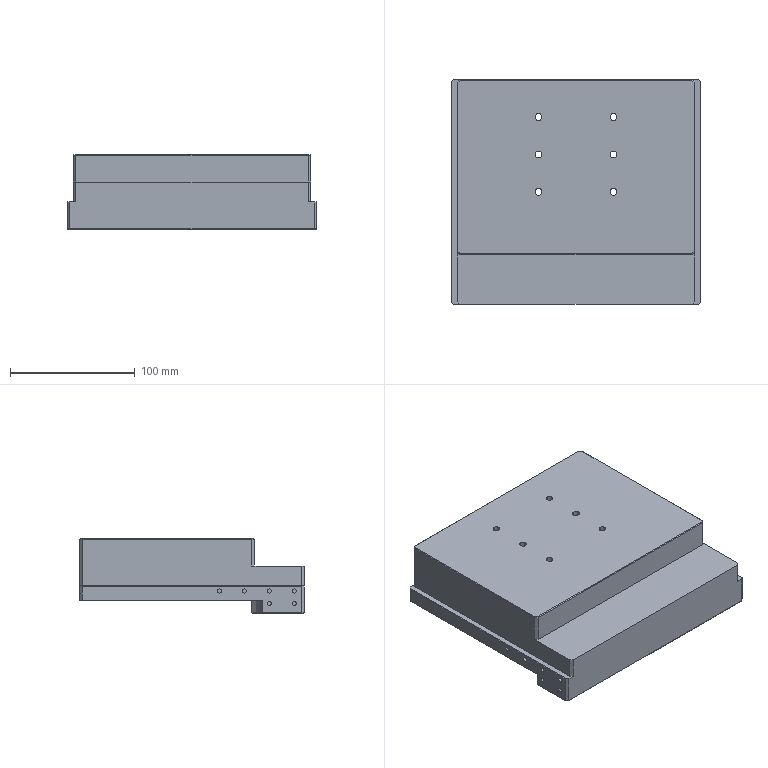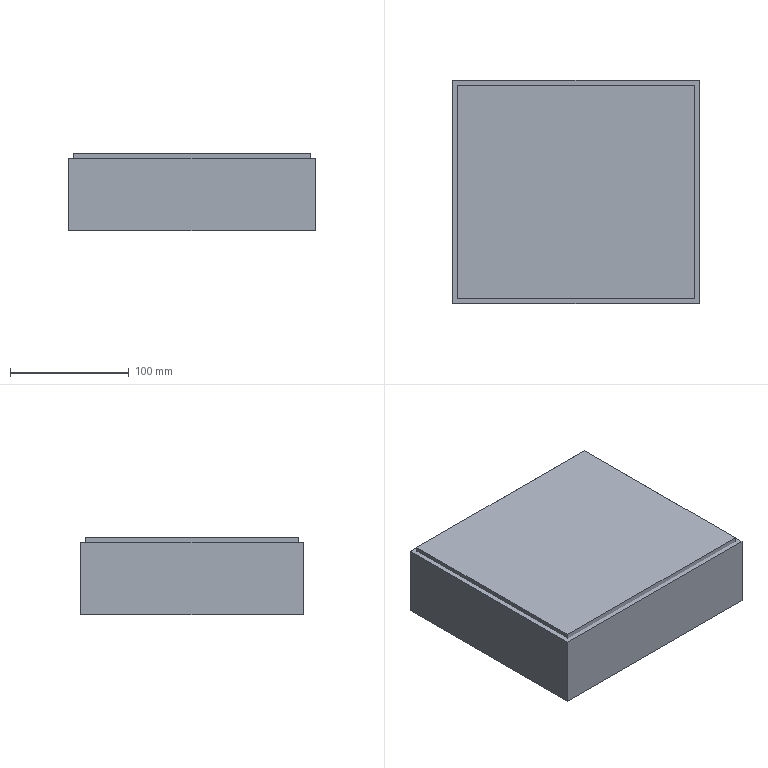CAM job | NX | 3-axis milling, drilling | part box 200 x 180 x 60 mm | stock box 208 x 188 x 65 mm
Tools:
number,name,description,diameter,corner_radius,flute_length,length,flutes
1,D63,Milling Tool-5 Parameters,63.0,0.0,50.0,75.0,2
7,D6A45,Milling Tool-5 Parameters,6.0,0.0,3.0,3.0,2
15,5.5ZT,Drilling Tool,5.5,0.0,35.0,50.0,2
20,D20,Milling Tool-5 Parameters,20.0,0.0,50.0,75.0,2
11,D10JING,Milling Tool-5 Parameters,10.0,0.0,50.0,75.0,2
10,D10,Milling Tool-5 Parameters,10.0,0.0,50.0,75.0,2
14,4.2ZT,Drilling Tool,4.2,0.0,35.0,50.0,2
15,M5,Milling Tool-5 Parameters,4.2,0.0,30.0,30.0,4
6,D6,Milling Tool-5 Parameters,6.0,0.0,50.0,75.0,2
Operations:
program,operation,operation_type,tool,method,geometry_group,spindle_rpm,surface_speed,feed_per_tooth,feed_cut,feed_plunge,cut_length_mm,path_length_mm,cut_time_min,machine_time_min
1-205-185-65毛胚,FLOOR_WALL,VolumeBased25DMillingOperation,D63,METHOD,A,6500.0,1286.0,0.0962,1250.0,100.0,1529.797,1583.797,1.224,1.229
1-205-185-65毛胚,DRILLING_COPY_1,Operation,D6A45,METHOD,A,3000.0,56.0,0.0333,200.0,0.0,27.6,310.873,0.138,0.1663
1-205-185-65毛胚,DRILLING_COPY_1_COPY_COPY_1_COPY_1,Operation,5.5ZT,METHOD,A,2000.0,41.0,0.075,120.0,0.0,327.914,911.502,2.733,2.791
1-205-185-65毛胚,CAVITY_MILL,CavityMilling,D20,METHOD,A,7000.0,439.0,0.1571,2200.0,1000.0,121807.808,129961.271,56.361,57.505
1-205-185-65毛胚,ZLEVEL_PROFILE_COPY_COPY_1,ZLevelMilling,D20,METHOD,A,7000.0,439.0,0.0571,800.0,100.0,1506.322,1626.905,1.883,1.895
1-205-185-65毛胚,ZLEVEL_PROFILE_COPY_COPY_1_COPY,ZLevelMilling,D20,METHOD,A,7000.0,439.0,0.0571,800.0,100.0,833.161,967.161,1.042,1.055
1-205-185-65毛胚,ZLEVEL_PROFILE_COPY_COPY_1_COPY_COPY,ZLevelMilling,D20,METHOD,A,7000.0,439.0,0.0571,800.0,100.0,1706.322,1902.905,2.133,2.153
1-205-185-65毛胚,FLOOR_WALL_1_COPY_1,VolumeBased25DMillingOperation,D20,METHOD,A,7000.0,87.0,0.0714,1000.0,100.0,1307.426,1723.342,1.307,1.349
1-205-185-65毛胚,ZLEVEL_PROFILE_COPY_1_COPY_COPY_COPY_COPY_2_COPY,ZLevelMilling,D6A45,METHOD,A,7000.0,131.0,0.0714,1000.0,1000.0,748.158,1609.378,0.7482,0.8343
1-205-185-65毛胚,ZLEVEL_PROFILE_COPY_1_COPY_COPY_COPY_COPY_2_COPY_COPY,ZLevelMilling,D6A45,METHOD,A,7000.0,131.0,0.0714,1000.0,1000.0,270.488,376.488,0.2705,0.2811
1-205-185-65毛胚,ZLEVEL_PROFILE_COPY_1_COPY_COPY_COPY_COPY_2_COPY_COPY_COPY,ZLevelMilling,D6A45,METHOD,A,7000.0,131.0,0.0714,1000.0,1000.0,394.18,862.643,0.3942,0.441
2-205-185-65毛胚,FLOOR_WALL_COPY,VolumeBased25DMillingOperation,D63,METHOD,B,6500.0,1286.0,0.0962,1250.0,100.0,7408.985,8900.425,5.927,6.076
2-205-185-65毛胚,FLOOR_WALL_1,VolumeBased25DMillingOperation,D10,METHOD,B,7000.0,219.0,0.1786,2500.0,1000.0,30183.498,30598.195,12.1,12.141
2-205-185-65毛胚,FLOOR_WALL_1_COPY,VolumeBased25DMillingOperation,D10,METHOD,B,7000.0,219.0,0.1786,2500.0,1000.0,1788.357,2636.707,0.7513,0.8362
2-205-185-65毛胚,DRILLING_COPY_1_COPY,Operation,D6A45,METHOD,B,3000.0,56.0,0.0333,200.0,0.0,134.4,1070.571,0.672,0.7656
2-205-185-65毛胚,DRILLING_COPY_1_COPY_1,Operation,4.2ZT,METHOD,B,2000.0,15.0,0.0375,150.0,0.0,490.712,1607.209,3.271,3.383
2-205-185-65毛胚,DRILLING_COPY_1_COPY_COPY,Operation,M5,METHOD,B,200.0,2.0,0.001,0.8,0.0,414.0,1453.784,517.5,517.604
2-205-185-65毛胚,FLOOR_WALL_1_COPY_1_COPY,VolumeBased25DMillingOperation,D10JING,METHOD,B,7000.0,87.0,0.0714,1000.0,100.0,6681.901,8337.026,6.682,6.848
2-205-185-65毛胚,HOLE_MILLING,CylinderMilling,D6,METHOD,B,7000.0,131.0,0.0857,1200.0,100.0,4414.197,5239.197,3.679,3.761
2-205-185-65毛胚,ZLEVEL_PROFILE_COPY_1_COPY_COPY_COPY_COPY_2_COPY_COPY_COPY_1,ZLevelMilling,D6A45,METHOD,B,7000.0,131.0,0.0714,1000.0,1000.0,573.346,1725.866,0.5733,0.6886
2-205-185-65毛胚,ZLEVEL_PROFILE_COPY_1_COPY_COPY_COPY_COPY_2_COPY_COPY_COPY_1_COPY,ZLevelMilling,D6A45,METHOD,B,7000.0,131.0,0.0714,1000.0,1000.0,783.301,3486.708,0.7833,1.054